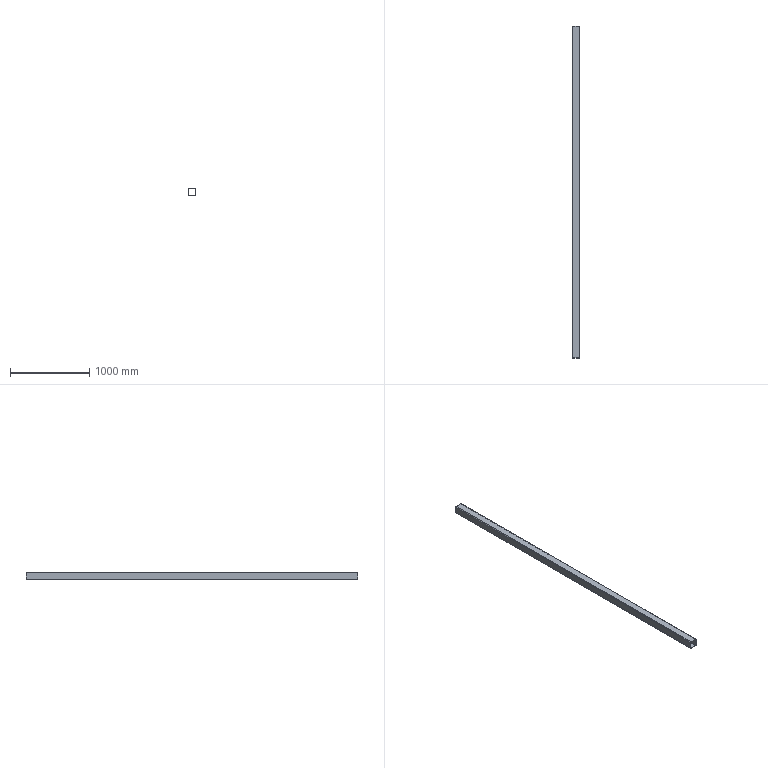Part | SolidWorks | features Extrusion 1 | 1 solid | 18 faces | box 100 x 4200 x 100 mm | volume 9836717 mm3 | plane 10 | cylinder 8 | commonest cylinder face diameters 12.6 x4 15.75 x4
STEP:
#1=CARTESIAN_POINT('',(100.,2100.,-90.6));
#2=VERTEX_POINT('',#1);
#3=CARTESIAN_POINT('',(92.125,2100.,-98.475));
#4=VERTEX_POINT('',#3);
#5=CARTESIAN_POINT('',(92.125,2100.,-90.6));
#6=DIRECTION('',(0.,1.,0.));
#7=DIRECTION('',(0.,0.,1.));
#8=AXIS2_PLACEMENT_3D('',#5,#6,#7);
#9=CIRCLE('',#8,7.875);
#10=EDGE_CURVE('',#2,#4,#9,.T.);
#11=ORIENTED_EDGE('',*,*,#10,.T.);
#12=CARTESIAN_POINT('',(7.875,2100.,-98.475));
#13=VERTEX_POINT('',#12);
#14=CARTESIAN_POINT('',(92.125,2100.,-98.475));
#15=DIRECTION('',(-1.,0.,0.));
#16=VECTOR('',#15,1000.);
#17=LINE('',#14,#16);
#18=EDGE_CURVE('',#4,#13,#17,.T.);
#19=ORIENTED_EDGE('',*,*,#18,.T.);
#20=CARTESIAN_POINT('',(0.,2100.,-90.6));
#21=VERTEX_POINT('',#20);
#22=CARTESIAN_POINT('',(7.875,2100.,-90.6));
#23=DIRECTION('',(0.,1.,0.));
#24=DIRECTION('',(0.,0.,1.));
#25=AXIS2_PLACEMENT_3D('',#22,#23,#24);
#26=CIRCLE('',#25,7.875);
#27=EDGE_CURVE('',#13,#21,#26,.T.);
#28=ORIENTED_EDGE('',*,*,#27,.T.);
#29=CARTESIAN_POINT('',(0.,2100.,-6.35));
#30=VERTEX_POINT('',#29);
#31=CARTESIAN_POINT('',(0.,2100.,-6.35));
#32=DIRECTION('',(0.,0.,1.));
#33=VECTOR('',#32,1000.);
#34=LINE('',#31,#33);
#35=EDGE_CURVE('',#21,#30,#34,.T.);
#36=ORIENTED_EDGE('',*,*,#35,.T.);
#37=CARTESIAN_POINT('',(7.875,2100.,1.525));
#38=VERTEX_POINT('',#37);
#39=CARTESIAN_POINT('',(7.875,2100.,-6.35));
#40=DIRECTION('',(0.,1.,0.));
#41=DIRECTION('',(0.,0.,1.));
#42=AXIS2_PLACEMENT_3D('',#39,#40,#41);
#43=CIRCLE('',#42,7.875);
#44=EDGE_CURVE('',#30,#38,#43,.T.);
#45=ORIENTED_EDGE('',*,*,#44,.T.);
#46=CARTESIAN_POINT('',(92.125,2100.,1.525));
#47=VERTEX_POINT('',#46);
#48=CARTESIAN_POINT('',(7.875,2100.,1.525));
#49=DIRECTION('',(1.,0.,0.));
#50=VECTOR('',#49,1000.);
#51=LINE('',#48,#50);
#52=EDGE_CURVE('',#38,#47,#51,.T.);
#53=ORIENTED_EDGE('',*,*,#52,.T.);
#54=CARTESIAN_POINT('',(100.,2100.,-6.35));
#55=VERTEX_POINT('',#54);
#56=CARTESIAN_POINT('',(92.125,2100.,-6.35));
#57=DIRECTION('',(0.,1.,0.));
#58=DIRECTION('',(0.,0.,1.));
#59=AXIS2_PLACEMENT_3D('',#56,#57,#58);
#60=CIRCLE('',#59,7.875);
#61=EDGE_CURVE('',#47,#55,#60,.T.);
#62=ORIENTED_EDGE('',*,*,#61,.T.);
#63=CARTESIAN_POINT('',(100.,2100.,-90.6));
#64=DIRECTION('',(0.,0.,-1.));
#65=VECTOR('',#64,1000.);
#66=LINE('',#63,#65);
#67=EDGE_CURVE('',#55,#2,#66,.T.);
#68=ORIENTED_EDGE('',*,*,#67,.T.);
#69=EDGE_LOOP('',(#11,#19,#28,#36,#45,#53,#62,#68));
#70=FACE_OUTER_BOUND('',#69,.T.);
#71=CARTESIAN_POINT('',(6.3,2100.,-85.875));
#72=VERTEX_POINT('',#71);
#73=CARTESIAN_POINT('',(6.3,2100.,-11.075));
#74=VERTEX_POINT('',#73);
#75=CARTESIAN_POINT('',(6.3,2100.,-11.075));
#76=DIRECTION('',(0.,0.,1.));
#77=VECTOR('',#76,1000.);
#78=LINE('',#75,#77);
#79=EDGE_CURVE('',#72,#74,#78,.T.);
#80=ORIENTED_EDGE('',*,*,#79,.F.);
#81=CARTESIAN_POINT('',(12.6,2100.,-92.175));
#82=VERTEX_POINT('',#81);
#83=CARTESIAN_POINT('',(12.6,2100.,-85.875));
#84=DIRECTION('',(0.,1.,0.));
#85=DIRECTION('',(0.,0.,1.));
#86=AXIS2_PLACEMENT_3D('',#83,#84,#85);
#87=CIRCLE('',#86,6.3);
#88=EDGE_CURVE('',#82,#72,#87,.T.);
#89=ORIENTED_EDGE('',*,*,#88,.F.);
#90=CARTESIAN_POINT('',(87.4,2100.,-92.175));
#91=VERTEX_POINT('',#90);
#92=CARTESIAN_POINT('',(87.4,2100.,-92.175));
#93=DIRECTION('',(-1.,0.,0.));
#94=VECTOR('',#93,1000.);
#95=LINE('',#92,#94);
#96=EDGE_CURVE('',#91,#82,#95,.T.);
#97=ORIENTED_EDGE('',*,*,#96,.F.);
#98=CARTESIAN_POINT('',(93.7,2100.,-85.875));
#99=VERTEX_POINT('',#98);
#100=CARTESIAN_POINT('',(87.4,2100.,-85.875));
#101=DIRECTION('',(0.,1.,0.));
#102=DIRECTION('',(0.,0.,1.));
#103=AXIS2_PLACEMENT_3D('',#100,#101,#102);
#104=CIRCLE('',#103,6.3);
#105=EDGE_CURVE('',#99,#91,#104,.T.);
#106=ORIENTED_EDGE('',*,*,#105,.F.);
#107=CARTESIAN_POINT('',(93.7,2100.,-11.075));
#108=VERTEX_POINT('',#107);
#109=CARTESIAN_POINT('',(93.7,2100.,-85.875));
#110=DIRECTION('',(0.,0.,-1.));
#111=VECTOR('',#110,1000.);
#112=LINE('',#109,#111);
#113=EDGE_CURVE('',#108,#99,#112,.T.);
#114=ORIENTED_EDGE('',*,*,#113,.F.);
#115=CARTESIAN_POINT('',(87.4,2100.,-4.775));
#116=VERTEX_POINT('',#115);
#117=CARTESIAN_POINT('',(87.4,2100.,-11.075));
#118=DIRECTION('',(0.,1.,0.));
#119=DIRECTION('',(0.,0.,1.));
#120=AXIS2_PLACEMENT_3D('',#117,#118,#119);
#121=CIRCLE('',#120,6.3);
#122=EDGE_CURVE('',#116,#108,#121,.T.);
#123=ORIENTED_EDGE('',*,*,#122,.F.);
#124=CARTESIAN_POINT('',(12.6,2100.,-4.775));
#125=VERTEX_POINT('',#124);
#126=CARTESIAN_POINT('',(12.6,2100.,-4.775));
#127=DIRECTION('',(1.,0.,0.));
#128=VECTOR('',#127,1000.);
#129=LINE('',#126,#128);
#130=EDGE_CURVE('',#125,#116,#129,.T.);
#131=ORIENTED_EDGE('',*,*,#130,.F.);
#132=CARTESIAN_POINT('',(12.6,2100.,-11.075));
#133=DIRECTION('',(0.,1.,0.));
#134=DIRECTION('',(0.,0.,1.));
#135=AXIS2_PLACEMENT_3D('',#132,#133,#134);
#136=CIRCLE('',#135,6.3);
#137=EDGE_CURVE('',#74,#125,#136,.T.);
#138=ORIENTED_EDGE('',*,*,#137,.F.);
#139=EDGE_LOOP('',(#80,#89,#97,#106,#114,#123,#131,#138));
#140=FACE_BOUND('',#139,.T.);
#141=CARTESIAN_POINT('',(92.125,2100.,-90.6));
#142=DIRECTION('',(0.,1.,0.));
#143=DIRECTION('',(0.,0.,1.));
#144=AXIS2_PLACEMENT_3D('',#141,#142,#143);
#145=PLANE('',#144);
#146=ADVANCED_FACE('',(#70,#140),#145,.T.);
#147=CARTESIAN_POINT('',(100.,-2100.,-90.6));
#148=VERTEX_POINT('',#147);
#149=CARTESIAN_POINT('',(92.125,-2100.,-98.475));
#150=VERTEX_POINT('',#149);
#151=CARTESIAN_POINT('',(92.125,-2100.,-90.6));
#152=DIRECTION('',(0.,1.,0.));
#153=DIRECTION('',(0.,0.,1.));
#154=AXIS2_PLACEMENT_3D('',#151,#152,#153);
#155=CIRCLE('',#154,7.875);
#156=EDGE_CURVE('',#148,#150,#155,.T.);
#157=ORIENTED_EDGE('',*,*,#156,.F.);
#158=CARTESIAN_POINT('',(100.,-2100.,-6.35));
#159=VERTEX_POINT('',#158);
#160=CARTESIAN_POINT('',(100.,-2100.,-90.6));
#161=DIRECTION('',(0.,0.,-1.));
#162=VECTOR('',#161,1000.);
#163=LINE('',#160,#162);
#164=EDGE_CURVE('',#159,#148,#163,.T.);
#165=ORIENTED_EDGE('',*,*,#164,.F.);
#166=CARTESIAN_POINT('',(92.125,-2100.,1.525));
#167=VERTEX_POINT('',#166);
#168=CARTESIAN_POINT('',(92.125,-2100.,-6.35));
#169=DIRECTION('',(0.,1.,0.));
#170=DIRECTION('',(0.,0.,1.));
#171=AXIS2_PLACEMENT_3D('',#168,#169,#170);
#172=CIRCLE('',#171,7.875);
#173=EDGE_CURVE('',#167,#159,#172,.T.);
#174=ORIENTED_EDGE('',*,*,#173,.F.);
#175=CARTESIAN_POINT('',(7.875,-2100.,1.525));
#176=VERTEX_POINT('',#175);
#177=CARTESIAN_POINT('',(7.875,-2100.,1.525));
#178=DIRECTION('',(1.,0.,0.));
#179=VECTOR('',#178,1000.);
#180=LINE('',#177,#179);
#181=EDGE_CURVE('',#176,#167,#180,.T.);
#182=ORIENTED_EDGE('',*,*,#181,.F.);
#183=CARTESIAN_POINT('',(0.,-2100.,-6.35));
#184=VERTEX_POINT('',#183);
#185=CARTESIAN_POINT('',(7.875,-2100.,-6.35));
#186=DIRECTION('',(0.,1.,0.));
#187=DIRECTION('',(0.,0.,1.));
#188=AXIS2_PLACEMENT_3D('',#185,#186,#187);
#189=CIRCLE('',#188,7.875);
#190=EDGE_CURVE('',#184,#176,#189,.T.);
#191=ORIENTED_EDGE('',*,*,#190,.F.);
#192=CARTESIAN_POINT('',(0.,-2100.,-90.6));
#193=VERTEX_POINT('',#192);
#194=CARTESIAN_POINT('',(0.,-2100.,-6.35));
#195=DIRECTION('',(0.,0.,1.));
#196=VECTOR('',#195,1000.);
#197=LINE('',#194,#196);
#198=EDGE_CURVE('',#193,#184,#197,.T.);
#199=ORIENTED_EDGE('',*,*,#198,.F.);
#200=CARTESIAN_POINT('',(7.875,-2100.,-98.475));
#201=VERTEX_POINT('',#200);
#202=CARTESIAN_POINT('',(7.875,-2100.,-90.6));
#203=DIRECTION('',(0.,1.,0.));
#204=DIRECTION('',(0.,0.,1.));
#205=AXIS2_PLACEMENT_3D('',#202,#203,#204);
#206=CIRCLE('',#205,7.875);
#207=EDGE_CURVE('',#201,#193,#206,.T.);
#208=ORIENTED_EDGE('',*,*,#207,.F.);
#209=CARTESIAN_POINT('',(92.125,-2100.,-98.475));
#210=DIRECTION('',(-1.,0.,0.));
#211=VECTOR('',#210,1000.);
#212=LINE('',#209,#211);
#213=EDGE_CURVE('',#150,#201,#212,.T.);
#214=ORIENTED_EDGE('',*,*,#213,.F.);
#215=EDGE_LOOP('',(#157,#165,#174,#182,#191,#199,#208,#214));
#216=FACE_OUTER_BOUND('',#215,.T.);
#217=CARTESIAN_POINT('',(12.6,-2100.,-92.175));
#218=VERTEX_POINT('',#217);
#219=CARTESIAN_POINT('',(6.3,-2100.,-85.875));
#220=VERTEX_POINT('',#219);
#221=CARTESIAN_POINT('',(12.6,-2100.,-85.875));
#222=DIRECTION('',(0.,1.,0.));
#223=DIRECTION('',(0.,0.,1.));
#224=AXIS2_PLACEMENT_3D('',#221,#222,#223);
#225=CIRCLE('',#224,6.3);
#226=EDGE_CURVE('',#218,#220,#225,.T.);
#227=ORIENTED_EDGE('',*,*,#226,.T.);
#228=CARTESIAN_POINT('',(6.3,-2100.,-11.075));
#229=VERTEX_POINT('',#228);
#230=CARTESIAN_POINT('',(6.3,-2100.,-11.075));
#231=DIRECTION('',(0.,0.,1.));
#232=VECTOR('',#231,1000.);
#233=LINE('',#230,#232);
#234=EDGE_CURVE('',#220,#229,#233,.T.);
#235=ORIENTED_EDGE('',*,*,#234,.T.);
#236=CARTESIAN_POINT('',(12.6,-2100.,-4.775));
#237=VERTEX_POINT('',#236);
#238=CARTESIAN_POINT('',(12.6,-2100.,-11.075));
#239=DIRECTION('',(0.,1.,0.));
#240=DIRECTION('',(0.,0.,1.));
#241=AXIS2_PLACEMENT_3D('',#238,#239,#240);
#242=CIRCLE('',#241,6.3);
#243=EDGE_CURVE('',#229,#237,#242,.T.);
#244=ORIENTED_EDGE('',*,*,#243,.T.);
#245=CARTESIAN_POINT('',(87.4,-2100.,-4.775));
#246=VERTEX_POINT('',#245);
#247=CARTESIAN_POINT('',(12.6,-2100.,-4.775));
#248=DIRECTION('',(1.,0.,0.));
#249=VECTOR('',#248,1000.);
#250=LINE('',#247,#249);
#251=EDGE_CURVE('',#237,#246,#250,.T.);
#252=ORIENTED_EDGE('',*,*,#251,.T.);
#253=CARTESIAN_POINT('',(93.7,-2100.,-11.075));
#254=VERTEX_POINT('',#253);
#255=CARTESIAN_POINT('',(87.4,-2100.,-11.075));
#256=DIRECTION('',(0.,1.,0.));
#257=DIRECTION('',(0.,0.,1.));
#258=AXIS2_PLACEMENT_3D('',#255,#256,#257);
#259=CIRCLE('',#258,6.3);
#260=EDGE_CURVE('',#246,#254,#259,.T.);
#261=ORIENTED_EDGE('',*,*,#260,.T.);
#262=CARTESIAN_POINT('',(93.7,-2100.,-85.875));
#263=VERTEX_POINT('',#262);
#264=CARTESIAN_POINT('',(93.7,-2100.,-85.875));
#265=DIRECTION('',(0.,0.,-1.));
#266=VECTOR('',#265,1000.);
#267=LINE('',#264,#266);
#268=EDGE_CURVE('',#254,#263,#267,.T.);
#269=ORIENTED_EDGE('',*,*,#268,.T.);
#270=CARTESIAN_POINT('',(87.4,-2100.,-92.175));
#271=VERTEX_POINT('',#270);
#272=CARTESIAN_POINT('',(87.4,-2100.,-85.875));
#273=DIRECTION('',(0.,1.,0.));
#274=DIRECTION('',(0.,0.,1.));
#275=AXIS2_PLACEMENT_3D('',#272,#273,#274);
#276=CIRCLE('',#275,6.3);
#277=EDGE_CURVE('',#263,#271,#276,.T.);
#278=ORIENTED_EDGE('',*,*,#277,.T.);
#279=CARTESIAN_POINT('',(87.4,-2100.,-92.175));
#280=DIRECTION('',(-1.,0.,0.));
#281=VECTOR('',#280,1000.);
#282=LINE('',#279,#281);
#283=EDGE_CURVE('',#271,#218,#282,.T.);
#284=ORIENTED_EDGE('',*,*,#283,.T.);
#285=EDGE_LOOP('',(#227,#235,#244,#252,#261,#269,#278,#284));
#286=FACE_BOUND('',#285,.T.);
#287=CARTESIAN_POINT('',(92.125,-2100.,-90.6));
#288=DIRECTION('',(0.,1.,0.));
#289=DIRECTION('',(0.,0.,1.));
#290=AXIS2_PLACEMENT_3D('',#287,#288,#289);
#291=PLANE('',#290);
#292=ADVANCED_FACE('',(#216,#286),#291,.F.);
#293=ORIENTED_EDGE('',*,*,#156,.T.);
#294=CARTESIAN_POINT('',(92.125,2100.,-98.475));
#295=DIRECTION('',(0.,-1.,0.));
#296=VECTOR('',#295,1000.);
#297=LINE('',#294,#296);
#298=EDGE_CURVE('',#4,#150,#297,.T.);
#299=ORIENTED_EDGE('',*,*,#298,.F.);
#300=ORIENTED_EDGE('',*,*,#10,.F.);
#301=CARTESIAN_POINT('',(100.,2100.,-90.6));
#302=DIRECTION('',(0.,-1.,0.));
#303=VECTOR('',#302,1000.);
#304=LINE('',#301,#303);
#305=EDGE_CURVE('',#2,#148,#304,.T.);
#306=ORIENTED_EDGE('',*,*,#305,.T.);
#307=EDGE_LOOP('',(#293,#299,#300,#306));
#308=FACE_OUTER_BOUND('',#307,.T.);
#309=CARTESIAN_POINT('',(92.125,2100.,-90.6));
#310=DIRECTION('',(0.,-1.,0.));
#311=DIRECTION('',(0.,0.,-1.));
#312=AXIS2_PLACEMENT_3D('',#309,#310,#311);
#313=CYLINDRICAL_SURFACE('',#312,7.875);
#314=ADVANCED_FACE('',(#308),#313,.T.);
#315=ORIENTED_EDGE('',*,*,#213,.T.);
#316=CARTESIAN_POINT('',(7.875,2100.,-98.475));
#317=DIRECTION('',(0.,-1.,0.));
#318=VECTOR('',#317,1000.);
#319=LINE('',#316,#318);
#320=EDGE_CURVE('',#13,#201,#319,.T.);
#321=ORIENTED_EDGE('',*,*,#320,.F.);
#322=ORIENTED_EDGE('',*,*,#18,.F.);
#323=ORIENTED_EDGE('',*,*,#298,.T.);
#324=EDGE_LOOP('',(#315,#321,#322,#323));
#325=FACE_OUTER_BOUND('',#324,.T.);
#326=CARTESIAN_POINT('',(92.125,2100.,-98.475));
#327=DIRECTION('',(0.,0.,1.));
#328=DIRECTION('',(1.,0.,0.));
#329=AXIS2_PLACEMENT_3D('',#326,#327,#328);
#330=PLANE('',#329);
#331=ADVANCED_FACE('',(#325),#330,.F.);
#332=ORIENTED_EDGE('',*,*,#207,.T.);
#333=CARTESIAN_POINT('',(0.,2100.,-90.6));
#334=DIRECTION('',(0.,-1.,0.));
#335=VECTOR('',#334,1000.);
#336=LINE('',#333,#335);
#337=EDGE_CURVE('',#21,#193,#336,.T.);
#338=ORIENTED_EDGE('',*,*,#337,.F.);
#339=ORIENTED_EDGE('',*,*,#27,.F.);
#340=ORIENTED_EDGE('',*,*,#320,.T.);
#341=EDGE_LOOP('',(#332,#338,#339,#340));
#342=FACE_OUTER_BOUND('',#341,.T.);
#343=CARTESIAN_POINT('',(7.875,2100.,-90.6));
#344=DIRECTION('',(0.,-1.,0.));
#345=DIRECTION('',(0.,0.,-1.));
#346=AXIS2_PLACEMENT_3D('',#343,#344,#345);
#347=CYLINDRICAL_SURFACE('',#346,7.875);
#348=ADVANCED_FACE('',(#342),#347,.T.);
#349=ORIENTED_EDGE('',*,*,#198,.T.);
#350=CARTESIAN_POINT('',(0.,2100.,-6.35));
#351=DIRECTION('',(0.,-1.,0.));
#352=VECTOR('',#351,1000.);
#353=LINE('',#350,#352);
#354=EDGE_CURVE('',#30,#184,#353,.T.);
#355=ORIENTED_EDGE('',*,*,#354,.F.);
#356=ORIENTED_EDGE('',*,*,#35,.F.);
#357=ORIENTED_EDGE('',*,*,#337,.T.);
#358=EDGE_LOOP('',(#349,#355,#356,#357));
#359=FACE_OUTER_BOUND('',#358,.T.);
#360=CARTESIAN_POINT('',(0.,2100.,-6.35));
#361=DIRECTION('',(1.,0.,0.));
#362=DIRECTION('',(0.,0.,-1.));
#363=AXIS2_PLACEMENT_3D('',#360,#361,#362);
#364=PLANE('',#363);
#365=ADVANCED_FACE('',(#359),#364,.F.);
#366=ORIENTED_EDGE('',*,*,#190,.T.);
#367=CARTESIAN_POINT('',(7.875,2100.,1.525));
#368=DIRECTION('',(0.,-1.,0.));
#369=VECTOR('',#368,1000.);
#370=LINE('',#367,#369);
#371=EDGE_CURVE('',#38,#176,#370,.T.);
#372=ORIENTED_EDGE('',*,*,#371,.F.);
#373=ORIENTED_EDGE('',*,*,#44,.F.);
#374=ORIENTED_EDGE('',*,*,#354,.T.);
#375=EDGE_LOOP('',(#366,#372,#373,#374));
#376=FACE_OUTER_BOUND('',#375,.T.);
#377=CARTESIAN_POINT('',(7.875,2100.,-6.35));
#378=DIRECTION('',(0.,-1.,0.));
#379=DIRECTION('',(0.,0.,-1.));
#380=AXIS2_PLACEMENT_3D('',#377,#378,#379);
#381=CYLINDRICAL_SURFACE('',#380,7.875);
#382=ADVANCED_FACE('',(#376),#381,.T.);
#383=ORIENTED_EDGE('',*,*,#181,.T.);
#384=CARTESIAN_POINT('',(92.125,2100.,1.525));
#385=DIRECTION('',(0.,-1.,0.));
#386=VECTOR('',#385,1000.);
#387=LINE('',#384,#386);
#388=EDGE_CURVE('',#47,#167,#387,.T.);
#389=ORIENTED_EDGE('',*,*,#388,.F.);
#390=ORIENTED_EDGE('',*,*,#52,.F.);
#391=ORIENTED_EDGE('',*,*,#371,.T.);
#392=EDGE_LOOP('',(#383,#389,#390,#391));
#393=FACE_OUTER_BOUND('',#392,.T.);
#394=CARTESIAN_POINT('',(7.875,2100.,1.525));
#395=DIRECTION('',(0.,0.,-1.));
#396=DIRECTION('',(-1.,0.,0.));
#397=AXIS2_PLACEMENT_3D('',#394,#395,#396);
#398=PLANE('',#397);
#399=ADVANCED_FACE('',(#393),#398,.F.);
#400=ORIENTED_EDGE('',*,*,#173,.T.);
#401=CARTESIAN_POINT('',(100.,2100.,-6.35));
#402=DIRECTION('',(0.,-1.,0.));
#403=VECTOR('',#402,1000.);
#404=LINE('',#401,#403);
#405=EDGE_CURVE('',#55,#159,#404,.T.);
#406=ORIENTED_EDGE('',*,*,#405,.F.);
#407=ORIENTED_EDGE('',*,*,#61,.F.);
#408=ORIENTED_EDGE('',*,*,#388,.T.);
#409=EDGE_LOOP('',(#400,#406,#407,#408));
#410=FACE_OUTER_BOUND('',#409,.T.);
#411=CARTESIAN_POINT('',(92.125,2100.,-6.35));
#412=DIRECTION('',(0.,-1.,0.));
#413=DIRECTION('',(0.,0.,-1.));
#414=AXIS2_PLACEMENT_3D('',#411,#412,#413);
#415=CYLINDRICAL_SURFACE('',#414,7.875);
#416=ADVANCED_FACE('',(#410),#415,.T.);
#417=ORIENTED_EDGE('',*,*,#164,.T.);
#418=ORIENTED_EDGE('',*,*,#305,.F.);
#419=ORIENTED_EDGE('',*,*,#67,.F.);
#420=ORIENTED_EDGE('',*,*,#405,.T.);
#421=EDGE_LOOP('',(#417,#418,#419,#420));
#422=FACE_OUTER_BOUND('',#421,.T.);
#423=CARTESIAN_POINT('',(100.,2100.,-90.6));
#424=DIRECTION('',(-1.,0.,0.));
#425=DIRECTION('',(0.,0.,1.));
#426=AXIS2_PLACEMENT_3D('',#423,#424,#425);
#427=PLANE('',#426);
#428=ADVANCED_FACE('',(#422),#427,.F.);
#429=ORIENTED_EDGE('',*,*,#226,.F.);
#430=CARTESIAN_POINT('',(12.6,2100.,-92.175));
#431=DIRECTION('',(0.,-1.,0.));
#432=VECTOR('',#431,1000.);
#433=LINE('',#430,#432);
#434=EDGE_CURVE('',#82,#218,#433,.T.);
#435=ORIENTED_EDGE('',*,*,#434,.F.);
#436=ORIENTED_EDGE('',*,*,#88,.T.);
#437=CARTESIAN_POINT('',(6.3,2100.,-85.875));
#438=DIRECTION('',(0.,-1.,0.));
#439=VECTOR('',#438,1000.);
#440=LINE('',#437,#439);
#441=EDGE_CURVE('',#72,#220,#440,.T.);
#442=ORIENTED_EDGE('',*,*,#441,.T.);
#443=EDGE_LOOP('',(#429,#435,#436,#442));
#444=FACE_OUTER_BOUND('',#443,.T.);
#445=CARTESIAN_POINT('',(12.6,2100.,-85.875));
#446=DIRECTION('',(0.,-1.,0.));
#447=DIRECTION('',(0.,0.,-1.));
#448=AXIS2_PLACEMENT_3D('',#445,#446,#447);
#449=CYLINDRICAL_SURFACE('',#448,6.3);
#450=ADVANCED_FACE('',(#444),#449,.F.);
#451=ORIENTED_EDGE('',*,*,#234,.F.);
#452=ORIENTED_EDGE('',*,*,#441,.F.);
#453=ORIENTED_EDGE('',*,*,#79,.T.);
#454=CARTESIAN_POINT('',(6.3,2100.,-11.075));
#455=DIRECTION('',(0.,-1.,0.));
#456=VECTOR('',#455,1000.);
#457=LINE('',#454,#456);
#458=EDGE_CURVE('',#74,#229,#457,.T.);
#459=ORIENTED_EDGE('',*,*,#458,.T.);
#460=EDGE_LOOP('',(#451,#452,#453,#459));
#461=FACE_OUTER_BOUND('',#460,.T.);
#462=CARTESIAN_POINT('',(6.3,2100.,-11.075));
#463=DIRECTION('',(1.,0.,0.));
#464=DIRECTION('',(0.,0.,-1.));
#465=AXIS2_PLACEMENT_3D('',#462,#463,#464);
#466=PLANE('',#465);
#467=ADVANCED_FACE('',(#461),#466,.T.);
#468=ORIENTED_EDGE('',*,*,#243,.F.);
#469=ORIENTED_EDGE('',*,*,#458,.F.);
#470=ORIENTED_EDGE('',*,*,#137,.T.);
#471=CARTESIAN_POINT('',(12.6,2100.,-4.775));
#472=DIRECTION('',(0.,-1.,0.));
#473=VECTOR('',#472,1000.);
#474=LINE('',#471,#473);
#475=EDGE_CURVE('',#125,#237,#474,.T.);
#476=ORIENTED_EDGE('',*,*,#475,.T.);
#477=EDGE_LOOP('',(#468,#469,#470,#476));
#478=FACE_OUTER_BOUND('',#477,.T.);
#479=CARTESIAN_POINT('',(12.6,2100.,-11.075));
#480=DIRECTION('',(0.,-1.,0.));
#481=DIRECTION('',(0.,0.,-1.));
#482=AXIS2_PLACEMENT_3D('',#479,#480,#481);
#483=CYLINDRICAL_SURFACE('',#482,6.3);
#484=ADVANCED_FACE('',(#478),#483,.F.);
#485=ORIENTED_EDGE('',*,*,#251,.F.);
#486=ORIENTED_EDGE('',*,*,#475,.F.);
#487=ORIENTED_EDGE('',*,*,#130,.T.);
#488=CARTESIAN_POINT('',(87.4,2100.,-4.775));
#489=DIRECTION('',(0.,-1.,0.));
#490=VECTOR('',#489,1000.);
#491=LINE('',#488,#490);
#492=EDGE_CURVE('',#116,#246,#491,.T.);
#493=ORIENTED_EDGE('',*,*,#492,.T.);
#494=EDGE_LOOP('',(#485,#486,#487,#493));
#495=FACE_OUTER_BOUND('',#494,.T.);
#496=CARTESIAN_POINT('',(12.6,2100.,-4.775));
#497=DIRECTION('',(0.,0.,-1.));
#498=DIRECTION('',(-1.,0.,0.));
#499=AXIS2_PLACEMENT_3D('',#496,#497,#498);
#500=PLANE('',#499);
#501=ADVANCED_FACE('',(#495),#500,.T.);
#502=ORIENTED_EDGE('',*,*,#260,.F.);
#503=ORIENTED_EDGE('',*,*,#492,.F.);
#504=ORIENTED_EDGE('',*,*,#122,.T.);
#505=CARTESIAN_POINT('',(93.7,2100.,-11.075));
#506=DIRECTION('',(0.,-1.,0.));
#507=VECTOR('',#506,1000.);
#508=LINE('',#505,#507);
#509=EDGE_CURVE('',#108,#254,#508,.T.);
#510=ORIENTED_EDGE('',*,*,#509,.T.);
#511=EDGE_LOOP('',(#502,#503,#504,#510));
#512=FACE_OUTER_BOUND('',#511,.T.);
#513=CARTESIAN_POINT('',(87.4,2100.,-11.075));
#514=DIRECTION('',(0.,-1.,0.));
#515=DIRECTION('',(0.,0.,-1.));
#516=AXIS2_PLACEMENT_3D('',#513,#514,#515);
#517=CYLINDRICAL_SURFACE('',#516,6.3);
#518=ADVANCED_FACE('',(#512),#517,.F.);
#519=ORIENTED_EDGE('',*,*,#268,.F.);
#520=ORIENTED_EDGE('',*,*,#509,.F.);
#521=ORIENTED_EDGE('',*,*,#113,.T.);
#522=CARTESIAN_POINT('',(93.7,2100.,-85.875));
#523=DIRECTION('',(0.,-1.,0.));
#524=VECTOR('',#523,1000.);
#525=LINE('',#522,#524);
#526=EDGE_CURVE('',#99,#263,#525,.T.);
#527=ORIENTED_EDGE('',*,*,#526,.T.);
#528=EDGE_LOOP('',(#519,#520,#521,#527));
#529=FACE_OUTER_BOUND('',#528,.T.);
#530=CARTESIAN_POINT('',(93.7,2100.,-85.875));
#531=DIRECTION('',(-1.,0.,0.));
#532=DIRECTION('',(0.,0.,1.));
#533=AXIS2_PLACEMENT_3D('',#530,#531,#532);
#534=PLANE('',#533);
#535=ADVANCED_FACE('',(#529),#534,.T.);
#536=ORIENTED_EDGE('',*,*,#277,.F.);
#537=ORIENTED_EDGE('',*,*,#526,.F.);
#538=ORIENTED_EDGE('',*,*,#105,.T.);
#539=CARTESIAN_POINT('',(87.4,2100.,-92.175));
#540=DIRECTION('',(0.,-1.,0.));
#541=VECTOR('',#540,1000.);
#542=LINE('',#539,#541);
#543=EDGE_CURVE('',#91,#271,#542,.T.);
#544=ORIENTED_EDGE('',*,*,#543,.T.);
#545=EDGE_LOOP('',(#536,#537,#538,#544));
#546=FACE_OUTER_BOUND('',#545,.T.);
#547=CARTESIAN_POINT('',(87.4,2100.,-85.875));
#548=DIRECTION('',(0.,-1.,0.));
#549=DIRECTION('',(0.,0.,-1.));
#550=AXIS2_PLACEMENT_3D('',#547,#548,#549);
#551=CYLINDRICAL_SURFACE('',#550,6.3);
#552=ADVANCED_FACE('',(#546),#551,.F.);
#553=ORIENTED_EDGE('',*,*,#283,.F.);
#554=ORIENTED_EDGE('',*,*,#543,.F.);
#555=ORIENTED_EDGE('',*,*,#96,.T.);
#556=ORIENTED_EDGE('',*,*,#434,.T.);
#557=EDGE_LOOP('',(#553,#554,#555,#556));
#558=FACE_OUTER_BOUND('',#557,.T.);
#559=CARTESIAN_POINT('',(87.4,2100.,-92.175));
#560=DIRECTION('',(0.,0.,1.));
#561=DIRECTION('',(1.,0.,0.));
#562=AXIS2_PLACEMENT_3D('',#559,#560,#561);
#563=PLANE('',#562);
#564=ADVANCED_FACE('',(#558),#563,.T.);
#565=CLOSED_SHELL('',(#146,#292,#314,#331,#348,#365,#382,#399,#416,#428,#450,#467,#484,#501,#518,#535,#552,#564));
#566=MANIFOLD_SOLID_BREP('',#565);
#567=CARTESIAN_POINT('',(0.,0.,0.));
#568=DIRECTION('',(0.,0.,1.));
#569=DIRECTION('',(1.,0.,0.));
#570=AXIS2_PLACEMENT_3D('',#567,#568,#569);
#571=(LENGTH_UNIT()NAMED_UNIT(*)SI_UNIT(.MILLI.,.METRE.));
#572=UNCERTAINTY_MEASURE_WITH_UNIT(LENGTH_MEASURE(0.00001),#571,'','');
#573=(NAMED_UNIT(*)PLANE_ANGLE_UNIT()SI_UNIT($,.RADIAN.));
#574=(NAMED_UNIT(*)SI_UNIT($,.STERADIAN.)SOLID_ANGLE_UNIT());
#575=(GEOMETRIC_REPRESENTATION_CONTEXT(3)GLOBAL_UNCERTAINTY_ASSIGNED_CONTEXT((#572))GLOBAL_UNIT_ASSIGNED_CONTEXT((#571,#573,#574))REPRESENTATION_CONTEXT('',''));
#576=ADVANCED_BREP_SHAPE_REPRESENTATION('',(#566,#570),#575);